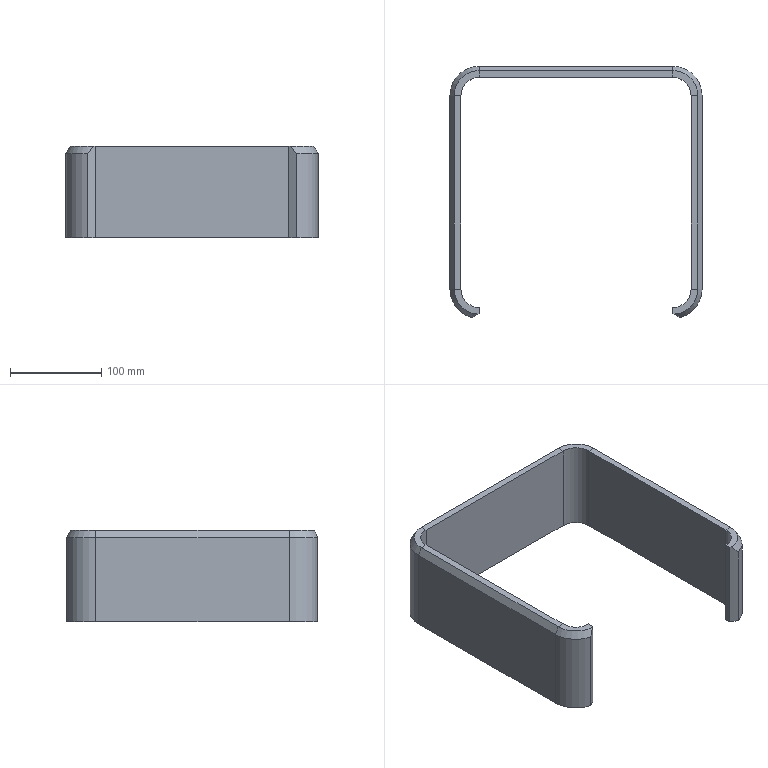Part | SolidWorks | features Chamfer 2, Extrusion 1, FlatPattern 1, RefAxis 1, SheetMetal 1, SolidToSheetMetal 1 | 1 solid | 39 faces | box 276 x 274.941 x 100 mm | volume 939173 mm3 | plane 27 | cylinder 8 | cone 4 | commonest cylinder face diameters 40 x4 64 x4
STEP:
#1=CARTESIAN_POINT('',(106.,-132.226,100.));
#2=VERTEX_POINT('',#1);
#3=CARTESIAN_POINT('',(106.,-126.,100.));
#4=VERTEX_POINT('',#3);
#5=CARTESIAN_POINT('',(106.,-126.,100.));
#6=DIRECTION('',(0.,1.,0.));
#7=VECTOR('',#6,1000.);
#8=LINE('',#5,#7);
#9=EDGE_CURVE('',#2,#4,#8,.T.);
#10=ORIENTED_EDGE('',*,*,#9,.F.);
#11=CARTESIAN_POINT('',(107.887,-133.316,100.));
#12=VERTEX_POINT('',#11);
#13=CARTESIAN_POINT('',(94.644,-125.67,100.));
#14=DIRECTION('',(0.866,-0.5,0.));
#15=VECTOR('',#14,1000.);
#16=LINE('',#13,#15);
#17=EDGE_CURVE('',#2,#12,#16,.T.);
#18=ORIENTED_EDGE('',*,*,#17,.T.);
#19=CARTESIAN_POINT('',(133.381,-106.,100.));
#20=VERTEX_POINT('',#19);
#21=CARTESIAN_POINT('',(106.,-106.,100.));
#22=DIRECTION('',(0.,0.,1.));
#23=DIRECTION('',(1.,0.,0.));
#24=AXIS2_PLACEMENT_3D('',#21,#22,#23);
#25=CIRCLE('',#24,27.381);
#26=EDGE_CURVE('',#12,#20,#25,.T.);
#27=ORIENTED_EDGE('',*,*,#26,.T.);
#28=CARTESIAN_POINT('',(126.,-106.,100.));
#29=VERTEX_POINT('',#28);
#30=CARTESIAN_POINT('',(126.,-106.,100.));
#31=DIRECTION('',(-1.,0.,0.));
#32=VECTOR('',#31,1000.);
#33=LINE('',#30,#32);
#34=EDGE_CURVE('',#20,#29,#33,.T.);
#35=ORIENTED_EDGE('',*,*,#34,.T.);
#36=CARTESIAN_POINT('',(106.,-106.,100.));
#37=DIRECTION('',(0.,0.,-1.));
#38=DIRECTION('',(1.,0.,0.));
#39=AXIS2_PLACEMENT_3D('',#36,#37,#38);
#40=CIRCLE('',#39,20.);
#41=EDGE_CURVE('',#29,#4,#40,.T.);
#42=ORIENTED_EDGE('',*,*,#41,.T.);
#43=EDGE_LOOP('',(#10,#18,#27,#35,#42));
#44=FACE_OUTER_BOUND('',#43,.T.);
#45=CARTESIAN_POINT('',(106.,-106.,100.));
#46=DIRECTION('',(0.,0.,1.));
#47=DIRECTION('',(1.,0.,0.));
#48=AXIS2_PLACEMENT_3D('',#45,#46,#47);
#49=PLANE('',#48);
#50=ADVANCED_FACE('',(#44),#49,.T.);
#51=ORIENTED_EDGE('',*,*,#34,.F.);
#52=CARTESIAN_POINT('',(133.381,106.,100.));
#53=VERTEX_POINT('',#52);
#54=CARTESIAN_POINT('',(133.381,106.,100.));
#55=DIRECTION('',(0.,1.,0.));
#56=VECTOR('',#55,1000.);
#57=LINE('',#54,#56);
#58=EDGE_CURVE('',#20,#53,#57,.T.);
#59=ORIENTED_EDGE('',*,*,#58,.T.);
#60=CARTESIAN_POINT('',(126.,106.,100.));
#61=VERTEX_POINT('',#60);
#62=CARTESIAN_POINT('',(126.,106.,100.));
#63=DIRECTION('',(-1.,0.,0.));
#64=VECTOR('',#63,1000.);
#65=LINE('',#62,#64);
#66=EDGE_CURVE('',#53,#61,#65,.T.);
#67=ORIENTED_EDGE('',*,*,#66,.T.);
#68=CARTESIAN_POINT('',(126.,106.,100.));
#69=DIRECTION('',(0.,-1.,0.));
#70=VECTOR('',#69,1000.);
#71=LINE('',#68,#70);
#72=EDGE_CURVE('',#61,#29,#71,.T.);
#73=ORIENTED_EDGE('',*,*,#72,.T.);
#74=EDGE_LOOP('',(#51,#59,#67,#73));
#75=FACE_OUTER_BOUND('',#74,.T.);
#76=CARTESIAN_POINT('',(126.,106.,100.));
#77=DIRECTION('',(0.,0.,1.));
#78=DIRECTION('',(0.,-1.,0.));
#79=AXIS2_PLACEMENT_3D('',#76,#77,#78);
#80=PLANE('',#79);
#81=ADVANCED_FACE('',(#75),#80,.T.);
#82=ORIENTED_EDGE('',*,*,#66,.F.);
#83=CARTESIAN_POINT('',(106.,133.381,100.));
#84=VERTEX_POINT('',#83);
#85=CARTESIAN_POINT('',(106.,106.,100.));
#86=DIRECTION('',(0.,0.,1.));
#87=DIRECTION('',(1.,0.,0.));
#88=AXIS2_PLACEMENT_3D('',#85,#86,#87);
#89=CIRCLE('',#88,27.381);
#90=EDGE_CURVE('',#53,#84,#89,.T.);
#91=ORIENTED_EDGE('',*,*,#90,.T.);
#92=CARTESIAN_POINT('',(106.,126.,100.));
#93=VERTEX_POINT('',#92);
#94=CARTESIAN_POINT('',(106.,126.,100.));
#95=DIRECTION('',(0.,-1.,0.));
#96=VECTOR('',#95,1000.);
#97=LINE('',#94,#96);
#98=EDGE_CURVE('',#84,#93,#97,.T.);
#99=ORIENTED_EDGE('',*,*,#98,.T.);
#100=CARTESIAN_POINT('',(106.,106.,100.));
#101=DIRECTION('',(0.,0.,-1.));
#102=DIRECTION('',(1.,0.,0.));
#103=AXIS2_PLACEMENT_3D('',#100,#101,#102);
#104=CIRCLE('',#103,20.);
#105=EDGE_CURVE('',#93,#61,#104,.T.);
#106=ORIENTED_EDGE('',*,*,#105,.T.);
#107=EDGE_LOOP('',(#82,#91,#99,#106));
#108=FACE_OUTER_BOUND('',#107,.T.);
#109=CARTESIAN_POINT('',(106.,106.,100.));
#110=DIRECTION('',(0.,0.,1.));
#111=DIRECTION('',(1.,0.,0.));
#112=AXIS2_PLACEMENT_3D('',#109,#110,#111);
#113=PLANE('',#112);
#114=ADVANCED_FACE('',(#108),#113,.T.);
#115=ORIENTED_EDGE('',*,*,#98,.F.);
#116=CARTESIAN_POINT('',(-106.,133.381,100.));
#117=VERTEX_POINT('',#116);
#118=CARTESIAN_POINT('',(-106.,133.381,100.));
#119=DIRECTION('',(-1.,0.,0.));
#120=VECTOR('',#119,1000.);
#121=LINE('',#118,#120);
#122=EDGE_CURVE('',#84,#117,#121,.T.);
#123=ORIENTED_EDGE('',*,*,#122,.T.);
#124=CARTESIAN_POINT('',(-106.,126.,100.));
#125=VERTEX_POINT('',#124);
#126=CARTESIAN_POINT('',(-106.,126.,100.));
#127=DIRECTION('',(0.,-1.,0.));
#128=VECTOR('',#127,1000.);
#129=LINE('',#126,#128);
#130=EDGE_CURVE('',#117,#125,#129,.T.);
#131=ORIENTED_EDGE('',*,*,#130,.T.);
#132=CARTESIAN_POINT('',(-106.,126.,100.));
#133=DIRECTION('',(1.,0.,0.));
#134=VECTOR('',#133,1000.);
#135=LINE('',#132,#134);
#136=EDGE_CURVE('',#125,#93,#135,.T.);
#137=ORIENTED_EDGE('',*,*,#136,.T.);
#138=EDGE_LOOP('',(#115,#123,#131,#137));
#139=FACE_OUTER_BOUND('',#138,.T.);
#140=CARTESIAN_POINT('',(-106.,126.,100.));
#141=DIRECTION('',(0.,0.,1.));
#142=DIRECTION('',(1.,0.,0.));
#143=AXIS2_PLACEMENT_3D('',#140,#141,#142);
#144=PLANE('',#143);
#145=ADVANCED_FACE('',(#139),#144,.T.);
#146=ORIENTED_EDGE('',*,*,#130,.F.);
#147=CARTESIAN_POINT('',(-133.381,106.,100.));
#148=VERTEX_POINT('',#147);
#149=CARTESIAN_POINT('',(-106.,106.,100.));
#150=DIRECTION('',(0.,0.,1.));
#151=DIRECTION('',(1.,0.,0.));
#152=AXIS2_PLACEMENT_3D('',#149,#150,#151);
#153=CIRCLE('',#152,27.381);
#154=EDGE_CURVE('',#117,#148,#153,.T.);
#155=ORIENTED_EDGE('',*,*,#154,.T.);
#156=CARTESIAN_POINT('',(-126.,106.,100.));
#157=VERTEX_POINT('',#156);
#158=CARTESIAN_POINT('',(-126.,106.,100.));
#159=DIRECTION('',(1.,0.,0.));
#160=VECTOR('',#159,1000.);
#161=LINE('',#158,#160);
#162=EDGE_CURVE('',#148,#157,#161,.T.);
#163=ORIENTED_EDGE('',*,*,#162,.T.);
#164=CARTESIAN_POINT('',(-106.,106.,100.));
#165=DIRECTION('',(0.,0.,-1.));
#166=DIRECTION('',(-1.,0.,0.));
#167=AXIS2_PLACEMENT_3D('',#164,#165,#166);
#168=CIRCLE('',#167,20.);
#169=EDGE_CURVE('',#157,#125,#168,.T.);
#170=ORIENTED_EDGE('',*,*,#169,.T.);
#171=EDGE_LOOP('',(#146,#155,#163,#170));
#172=FACE_OUTER_BOUND('',#171,.T.);
#173=CARTESIAN_POINT('',(-106.,106.,100.));
#174=DIRECTION('',(0.,0.,1.));
#175=DIRECTION('',(1.,0.,0.));
#176=AXIS2_PLACEMENT_3D('',#173,#174,#175);
#177=PLANE('',#176);
#178=ADVANCED_FACE('',(#172),#177,.T.);
#179=ORIENTED_EDGE('',*,*,#162,.F.);
#180=CARTESIAN_POINT('',(-133.381,-106.,100.));
#181=VERTEX_POINT('',#180);
#182=CARTESIAN_POINT('',(-133.381,-62.,100.));
#183=DIRECTION('',(0.,-1.,0.));
#184=VECTOR('',#183,1000.);
#185=LINE('',#182,#184);
#186=EDGE_CURVE('',#148,#181,#185,.T.);
#187=ORIENTED_EDGE('',*,*,#186,.T.);
#188=CARTESIAN_POINT('',(-126.,-106.,100.));
#189=VERTEX_POINT('',#188);
#190=CARTESIAN_POINT('',(-126.,-106.,100.));
#191=DIRECTION('',(1.,0.,0.));
#192=VECTOR('',#191,1000.);
#193=LINE('',#190,#192);
#194=EDGE_CURVE('',#181,#189,#193,.T.);
#195=ORIENTED_EDGE('',*,*,#194,.T.);
#196=CARTESIAN_POINT('',(-126.,-62.,100.));
#197=DIRECTION('',(0.,1.,0.));
#198=VECTOR('',#197,1000.);
#199=LINE('',#196,#198);
#200=EDGE_CURVE('',#189,#157,#199,.T.);
#201=ORIENTED_EDGE('',*,*,#200,.T.);
#202=EDGE_LOOP('',(#179,#187,#195,#201));
#203=FACE_OUTER_BOUND('',#202,.T.);
#204=CARTESIAN_POINT('',(-126.,-62.,100.));
#205=DIRECTION('',(0.,0.,1.));
#206=DIRECTION('',(0.,1.,0.));
#207=AXIS2_PLACEMENT_3D('',#204,#205,#206);
#208=PLANE('',#207);
#209=ADVANCED_FACE('',(#203),#208,.T.);
#210=CARTESIAN_POINT('',(-107.887,-133.316,100.));
#211=VERTEX_POINT('',#210);
#212=CARTESIAN_POINT('',(-106.,-106.,100.));
#213=DIRECTION('',(0.,0.,1.));
#214=DIRECTION('',(1.,0.,0.));
#215=AXIS2_PLACEMENT_3D('',#212,#213,#214);
#216=CIRCLE('',#215,27.381);
#217=EDGE_CURVE('',#181,#211,#216,.T.);
#218=ORIENTED_EDGE('',*,*,#217,.T.);
#219=CARTESIAN_POINT('',(-106.,-132.226,100.));
#220=VERTEX_POINT('',#219);
#221=CARTESIAN_POINT('',(-94.644,-125.67,100.));
#222=DIRECTION('',(0.866,0.5,0.));
#223=VECTOR('',#222,1000.);
#224=LINE('',#221,#223);
#225=EDGE_CURVE('',#211,#220,#224,.T.);
#226=ORIENTED_EDGE('',*,*,#225,.T.);
#227=CARTESIAN_POINT('',(-106.,-126.,100.));
#228=VERTEX_POINT('',#227);
#229=CARTESIAN_POINT('',(-106.,-126.,100.));
#230=DIRECTION('',(0.,1.,0.));
#231=VECTOR('',#230,1000.);
#232=LINE('',#229,#231);
#233=EDGE_CURVE('',#220,#228,#232,.T.);
#234=ORIENTED_EDGE('',*,*,#233,.T.);
#235=CARTESIAN_POINT('',(-106.,-106.,100.));
#236=DIRECTION('',(0.,0.,-1.));
#237=DIRECTION('',(-1.,0.,0.));
#238=AXIS2_PLACEMENT_3D('',#235,#236,#237);
#239=CIRCLE('',#238,20.);
#240=EDGE_CURVE('',#228,#189,#239,.T.);
#241=ORIENTED_EDGE('',*,*,#240,.T.);
#242=ORIENTED_EDGE('',*,*,#194,.F.);
#243=EDGE_LOOP('',(#218,#226,#234,#241,#242));
#244=FACE_OUTER_BOUND('',#243,.T.);
#245=CARTESIAN_POINT('',(-106.,-106.,100.));
#246=DIRECTION('',(0.,0.,1.));
#247=DIRECTION('',(1.,0.,0.));
#248=AXIS2_PLACEMENT_3D('',#245,#246,#247);
#249=PLANE('',#248);
#250=ADVANCED_FACE('',(#244),#249,.T.);
#251=ORIENTED_EDGE('',*,*,#233,.F.);
#252=CARTESIAN_POINT('',(-106.,-132.226,0.));
#253=VERTEX_POINT('',#252);
#254=CARTESIAN_POINT('',(-106.,-132.226,50.));
#255=DIRECTION('',(0.,0.,-1.));
#256=VECTOR('',#255,1000.);
#257=LINE('',#254,#256);
#258=EDGE_CURVE('',#220,#253,#257,.T.);
#259=ORIENTED_EDGE('',*,*,#258,.T.);
#260=CARTESIAN_POINT('',(-106.,-126.,0.));
#261=VERTEX_POINT('',#260);
#262=CARTESIAN_POINT('',(-106.,-126.,0.));
#263=DIRECTION('',(0.,1.,0.));
#264=VECTOR('',#263,1000.);
#265=LINE('',#262,#264);
#266=EDGE_CURVE('',#253,#261,#265,.T.);
#267=ORIENTED_EDGE('',*,*,#266,.T.);
#268=CARTESIAN_POINT('',(-106.,-126.,100.));
#269=DIRECTION('',(0.,0.,-1.));
#270=VECTOR('',#269,1000.);
#271=LINE('',#268,#270);
#272=EDGE_CURVE('',#228,#261,#271,.T.);
#273=ORIENTED_EDGE('',*,*,#272,.F.);
#274=EDGE_LOOP('',(#251,#259,#267,#273));
#275=FACE_OUTER_BOUND('',#274,.T.);
#276=CARTESIAN_POINT('',(-106.,-126.,50.));
#277=DIRECTION('',(-1.,0.,0.));
#278=DIRECTION('',(0.,0.,-1.));
#279=AXIS2_PLACEMENT_3D('',#276,#277,#278);
#280=PLANE('',#279);
#281=ADVANCED_FACE('',(#275),#280,.F.);
#282=ORIENTED_EDGE('',*,*,#266,.F.);
#283=CARTESIAN_POINT('',(-114.165,-136.941,0.));
#284=VERTEX_POINT('',#283);
#285=CARTESIAN_POINT('',(-94.644,-125.67,0.));
#286=DIRECTION('',(-0.866,-0.5,0.));
#287=VECTOR('',#286,1000.);
#288=LINE('',#285,#287);
#289=EDGE_CURVE('',#253,#284,#288,.T.);
#290=ORIENTED_EDGE('',*,*,#289,.T.);
#291=CARTESIAN_POINT('',(-138.,-106.,0.));
#292=VERTEX_POINT('',#291);
#293=CARTESIAN_POINT('',(-106.,-106.,0.));
#294=DIRECTION('',(0.,0.,-1.));
#295=DIRECTION('',(-1.,0.,0.));
#296=AXIS2_PLACEMENT_3D('',#293,#294,#295);
#297=CIRCLE('',#296,32.);
#298=EDGE_CURVE('',#284,#292,#297,.T.);
#299=ORIENTED_EDGE('',*,*,#298,.T.);
#300=CARTESIAN_POINT('',(-126.,-106.,0.));
#301=VERTEX_POINT('',#300);
#302=CARTESIAN_POINT('',(-126.,-106.,0.));
#303=DIRECTION('',(1.,0.,0.));
#304=VECTOR('',#303,1000.);
#305=LINE('',#302,#304);
#306=EDGE_CURVE('',#292,#301,#305,.T.);
#307=ORIENTED_EDGE('',*,*,#306,.T.);
#308=CARTESIAN_POINT('',(-106.,-106.,0.));
#309=DIRECTION('',(0.,0.,-1.));
#310=DIRECTION('',(-1.,0.,0.));
#311=AXIS2_PLACEMENT_3D('',#308,#309,#310);
#312=CIRCLE('',#311,20.);
#313=EDGE_CURVE('',#261,#301,#312,.T.);
#314=ORIENTED_EDGE('',*,*,#313,.F.);
#315=EDGE_LOOP('',(#282,#290,#299,#307,#314));
#316=FACE_OUTER_BOUND('',#315,.T.);
#317=CARTESIAN_POINT('',(-106.,-106.,0.));
#318=DIRECTION('',(0.,0.,1.));
#319=DIRECTION('',(1.,0.,0.));
#320=AXIS2_PLACEMENT_3D('',#317,#318,#319);
#321=PLANE('',#320);
#322=ADVANCED_FACE('',(#316),#321,.F.);
#323=ORIENTED_EDGE('',*,*,#306,.F.);
#324=CARTESIAN_POINT('',(-138.,106.,0.));
#325=VERTEX_POINT('',#324);
#326=CARTESIAN_POINT('',(-138.,106.,0.));
#327=DIRECTION('',(0.,1.,0.));
#328=VECTOR('',#327,1000.);
#329=LINE('',#326,#328);
#330=EDGE_CURVE('',#292,#325,#329,.T.);
#331=ORIENTED_EDGE('',*,*,#330,.T.);
#332=CARTESIAN_POINT('',(-126.,106.,0.));
#333=VERTEX_POINT('',#332);
#334=CARTESIAN_POINT('',(-126.,106.,0.));
#335=DIRECTION('',(1.,0.,0.));
#336=VECTOR('',#335,1000.);
#337=LINE('',#334,#336);
#338=EDGE_CURVE('',#325,#333,#337,.T.);
#339=ORIENTED_EDGE('',*,*,#338,.T.);
#340=CARTESIAN_POINT('',(-126.,106.,0.));
#341=DIRECTION('',(0.,1.,0.));
#342=VECTOR('',#341,1000.);
#343=LINE('',#340,#342);
#344=EDGE_CURVE('',#301,#333,#343,.T.);
#345=ORIENTED_EDGE('',*,*,#344,.F.);
#346=EDGE_LOOP('',(#323,#331,#339,#345));
#347=FACE_OUTER_BOUND('',#346,.T.);
#348=CARTESIAN_POINT('',(-126.,106.,0.));
#349=DIRECTION('',(0.,0.,1.));
#350=DIRECTION('',(0.,1.,0.));
#351=AXIS2_PLACEMENT_3D('',#348,#349,#350);
#352=PLANE('',#351);
#353=ADVANCED_FACE('',(#347),#352,.F.);
#354=ORIENTED_EDGE('',*,*,#338,.F.);
#355=CARTESIAN_POINT('',(-106.,138.,0.));
#356=VERTEX_POINT('',#355);
#357=CARTESIAN_POINT('',(-106.,106.,0.));
#358=DIRECTION('',(0.,0.,-1.));
#359=DIRECTION('',(-1.,0.,0.));
#360=AXIS2_PLACEMENT_3D('',#357,#358,#359);
#361=CIRCLE('',#360,32.);
#362=EDGE_CURVE('',#325,#356,#361,.T.);
#363=ORIENTED_EDGE('',*,*,#362,.T.);
#364=CARTESIAN_POINT('',(-106.,126.,0.));
#365=VERTEX_POINT('',#364);
#366=CARTESIAN_POINT('',(-106.,126.,0.));
#367=DIRECTION('',(0.,-1.,0.));
#368=VECTOR('',#367,1000.);
#369=LINE('',#366,#368);
#370=EDGE_CURVE('',#356,#365,#369,.T.);
#371=ORIENTED_EDGE('',*,*,#370,.T.);
#372=CARTESIAN_POINT('',(-106.,106.,0.));
#373=DIRECTION('',(0.,0.,-1.));
#374=DIRECTION('',(-1.,0.,0.));
#375=AXIS2_PLACEMENT_3D('',#372,#373,#374);
#376=CIRCLE('',#375,20.);
#377=EDGE_CURVE('',#333,#365,#376,.T.);
#378=ORIENTED_EDGE('',*,*,#377,.F.);
#379=EDGE_LOOP('',(#354,#363,#371,#378));
#380=FACE_OUTER_BOUND('',#379,.T.);
#381=CARTESIAN_POINT('',(-106.,106.,0.));
#382=DIRECTION('',(0.,0.,1.));
#383=DIRECTION('',(1.,0.,0.));
#384=AXIS2_PLACEMENT_3D('',#381,#382,#383);
#385=PLANE('',#384);
#386=ADVANCED_FACE('',(#380),#385,.F.);
#387=ORIENTED_EDGE('',*,*,#370,.F.);
#388=CARTESIAN_POINT('',(106.,138.,0.));
#389=VERTEX_POINT('',#388);
#390=CARTESIAN_POINT('',(-106.,138.,0.));
#391=DIRECTION('',(1.,0.,0.));
#392=VECTOR('',#391,1000.);
#393=LINE('',#390,#392);
#394=EDGE_CURVE('',#356,#389,#393,.T.);
#395=ORIENTED_EDGE('',*,*,#394,.T.);
#396=CARTESIAN_POINT('',(106.,126.,0.));
#397=VERTEX_POINT('',#396);
#398=CARTESIAN_POINT('',(106.,126.,0.));
#399=DIRECTION('',(0.,-1.,0.));
#400=VECTOR('',#399,1000.);
#401=LINE('',#398,#400);
#402=EDGE_CURVE('',#389,#397,#401,.T.);
#403=ORIENTED_EDGE('',*,*,#402,.T.);
#404=CARTESIAN_POINT('',(-106.,126.,0.));
#405=DIRECTION('',(1.,0.,0.));
#406=VECTOR('',#405,1000.);
#407=LINE('',#404,#406);
#408=EDGE_CURVE('',#365,#397,#407,.T.);
#409=ORIENTED_EDGE('',*,*,#408,.F.);
#410=EDGE_LOOP('',(#387,#395,#403,#409));
#411=FACE_OUTER_BOUND('',#410,.T.);
#412=CARTESIAN_POINT('',(-106.,126.,0.));
#413=DIRECTION('',(0.,0.,1.));
#414=DIRECTION('',(1.,0.,0.));
#415=AXIS2_PLACEMENT_3D('',#412,#413,#414);
#416=PLANE('',#415);
#417=ADVANCED_FACE('',(#411),#416,.F.);
#418=ORIENTED_EDGE('',*,*,#402,.F.);
#419=CARTESIAN_POINT('',(138.,106.,0.));
#420=VERTEX_POINT('',#419);
#421=CARTESIAN_POINT('',(106.,106.,0.));
#422=DIRECTION('',(0.,0.,-1.));
#423=DIRECTION('',(-1.,0.,0.));
#424=AXIS2_PLACEMENT_3D('',#421,#422,#423);
#425=CIRCLE('',#424,32.);
#426=EDGE_CURVE('',#389,#420,#425,.T.);
#427=ORIENTED_EDGE('',*,*,#426,.T.);
#428=CARTESIAN_POINT('',(126.,106.,0.));
#429=VERTEX_POINT('',#428);
#430=CARTESIAN_POINT('',(126.,106.,0.));
#431=DIRECTION('',(-1.,0.,0.));
#432=VECTOR('',#431,1000.);
#433=LINE('',#430,#432);
#434=EDGE_CURVE('',#420,#429,#433,.T.);
#435=ORIENTED_EDGE('',*,*,#434,.T.);
#436=CARTESIAN_POINT('',(106.,106.,0.));
#437=DIRECTION('',(0.,0.,-1.));
#438=DIRECTION('',(1.,0.,0.));
#439=AXIS2_PLACEMENT_3D('',#436,#437,#438);
#440=CIRCLE('',#439,20.);
#441=EDGE_CURVE('',#397,#429,#440,.T.);
#442=ORIENTED_EDGE('',*,*,#441,.F.);
#443=EDGE_LOOP('',(#418,#427,#435,#442));
#444=FACE_OUTER_BOUND('',#443,.T.);
#445=CARTESIAN_POINT('',(106.,106.,0.));
#446=DIRECTION('',(0.,0.,1.));
#447=DIRECTION('',(1.,0.,0.));
#448=AXIS2_PLACEMENT_3D('',#445,#446,#447);
#449=PLANE('',#448);
#450=ADVANCED_FACE('',(#444),#449,.F.);
#451=ORIENTED_EDGE('',*,*,#434,.F.);
#452=CARTESIAN_POINT('',(138.,-106.,0.));
#453=VERTEX_POINT('',#452);
#454=CARTESIAN_POINT('',(138.,-106.,0.));
#455=DIRECTION('',(0.,-1.,0.));
#456=VECTOR('',#455,1000.);
#457=LINE('',#454,#456);
#458=EDGE_CURVE('',#420,#453,#457,.T.);
#459=ORIENTED_EDGE('',*,*,#458,.T.);
#460=CARTESIAN_POINT('',(126.,-106.,0.));
#461=VERTEX_POINT('',#460);
#462=CARTESIAN_POINT('',(126.,-106.,0.));
#463=DIRECTION('',(-1.,0.,0.));
#464=VECTOR('',#463,1000.);
#465=LINE('',#462,#464);
#466=EDGE_CURVE('',#453,#461,#465,.T.);
#467=ORIENTED_EDGE('',*,*,#466,.T.);
#468=CARTESIAN_POINT('',(126.,-106.,0.));
#469=DIRECTION('',(0.,-1.,0.));
#470=VECTOR('',#469,1000.);
#471=LINE('',#468,#470);
#472=EDGE_CURVE('',#429,#461,#471,.T.);
#473=ORIENTED_EDGE('',*,*,#472,.F.);
#474=EDGE_LOOP('',(#451,#459,#467,#473));
#475=FACE_OUTER_BOUND('',#474,.T.);
#476=CARTESIAN_POINT('',(126.,-106.,0.));
#477=DIRECTION('',(0.,0.,1.));
#478=DIRECTION('',(0.,-1.,0.));
#479=AXIS2_PLACEMENT_3D('',#476,#477,#478);
#480=PLANE('',#479);
#481=ADVANCED_FACE('',(#475),#480,.F.);
#482=CARTESIAN_POINT('',(114.165,-136.941,0.));
#483=VERTEX_POINT('',#482);
#484=CARTESIAN_POINT('',(106.,-106.,0.));
#485=DIRECTION('',(0.,0.,-1.));
#486=DIRECTION('',(-1.,0.,0.));
#487=AXIS2_PLACEMENT_3D('',#484,#485,#486);
#488=CIRCLE('',#487,32.);
#489=EDGE_CURVE('',#453,#483,#488,.T.);
#490=ORIENTED_EDGE('',*,*,#489,.T.);
#491=CARTESIAN_POINT('',(106.,-132.226,0.));
#492=VERTEX_POINT('',#491);
#493=CARTESIAN_POINT('',(94.644,-125.67,0.));
#494=DIRECTION('',(-0.866,0.5,0.));
#495=VECTOR('',#494,1000.);
#496=LINE('',#493,#495);
#497=EDGE_CURVE('',#483,#492,#496,.T.);
#498=ORIENTED_EDGE('',*,*,#497,.T.);
#499=CARTESIAN_POINT('',(106.,-126.,0.));
#500=VERTEX_POINT('',#499);
#501=CARTESIAN_POINT('',(106.,-126.,0.));
#502=DIRECTION('',(0.,1.,0.));
#503=VECTOR('',#502,1000.);
#504=LINE('',#501,#503);
#505=EDGE_CURVE('',#492,#500,#504,.T.);
#506=ORIENTED_EDGE('',*,*,#505,.T.);
#507=CARTESIAN_POINT('',(106.,-106.,0.));
#508=DIRECTION('',(0.,0.,-1.));
#509=DIRECTION('',(1.,0.,0.));
#510=AXIS2_PLACEMENT_3D('',#507,#508,#509);
#511=CIRCLE('',#510,20.);
#512=EDGE_CURVE('',#461,#500,#511,.T.);
#513=ORIENTED_EDGE('',*,*,#512,.F.);
#514=ORIENTED_EDGE('',*,*,#466,.F.);
#515=EDGE_LOOP('',(#490,#498,#506,#513,#514));
#516=FACE_OUTER_BOUND('',#515,.T.);
#517=CARTESIAN_POINT('',(106.,-106.,0.));
#518=DIRECTION('',(0.,0.,1.));
#519=DIRECTION('',(1.,0.,0.));
#520=AXIS2_PLACEMENT_3D('',#517,#518,#519);
#521=PLANE('',#520);
#522=ADVANCED_FACE('',(#516),#521,.F.);
#523=ORIENTED_EDGE('',*,*,#505,.F.);
#524=CARTESIAN_POINT('',(106.,-132.226,50.));
#525=DIRECTION('',(0.,0.,1.));
#526=VECTOR('',#525,1000.);
#527=LINE('',#524,#526);
#528=EDGE_CURVE('',#492,#2,#527,.T.);
#529=ORIENTED_EDGE('',*,*,#528,.T.);
#530=ORIENTED_EDGE('',*,*,#9,.T.);
#531=CARTESIAN_POINT('',(106.,-126.,100.));
#532=DIRECTION('',(0.,0.,-1.));
#533=VECTOR('',#532,1000.);
#534=LINE('',#531,#533);
#535=EDGE_CURVE('',#4,#500,#534,.T.);
#536=ORIENTED_EDGE('',*,*,#535,.T.);
#537=EDGE_LOOP('',(#523,#529,#530,#536));
#538=FACE_OUTER_BOUND('',#537,.T.);
#539=CARTESIAN_POINT('',(106.,-126.,50.));
#540=DIRECTION('',(-1.,0.,0.));
#541=DIRECTION('',(0.,0.,-1.));
#542=AXIS2_PLACEMENT_3D('',#539,#540,#541);
#543=PLANE('',#542);
#544=ADVANCED_FACE('',(#538),#543,.T.);
#545=ORIENTED_EDGE('',*,*,#512,.T.);
#546=ORIENTED_EDGE('',*,*,#535,.F.);
#547=ORIENTED_EDGE('',*,*,#41,.F.);
#548=CARTESIAN_POINT('',(126.,-106.,100.));
#549=DIRECTION('',(0.,0.,-1.));
#550=VECTOR('',#549,1000.);
#551=LINE('',#548,#550);
#552=EDGE_CURVE('',#29,#461,#551,.T.);
#553=ORIENTED_EDGE('',*,*,#552,.T.);
#554=EDGE_LOOP('',(#545,#546,#547,#553));
#555=FACE_OUTER_BOUND('',#554,.T.);
#556=CARTESIAN_POINT('',(106.,-106.,100.));
#557=DIRECTION('',(0.,0.,-1.));
#558=DIRECTION('',(-1.,0.,0.));
#559=AXIS2_PLACEMENT_3D('',#556,#557,#558);
#560=CYLINDRICAL_SURFACE('',#559,20.);
#561=ADVANCED_FACE('',(#555),#560,.F.);
#562=ORIENTED_EDGE('',*,*,#313,.T.);
#563=CARTESIAN_POINT('',(-126.,-106.,100.));
#564=DIRECTION('',(0.,0.,-1.));
#565=VECTOR('',#564,1000.);
#566=LINE('',#563,#565);
#567=EDGE_CURVE('',#189,#301,#566,.T.);
#568=ORIENTED_EDGE('',*,*,#567,.F.);
#569=ORIENTED_EDGE('',*,*,#240,.F.);
#570=ORIENTED_EDGE('',*,*,#272,.T.);
#571=EDGE_LOOP('',(#562,#568,#569,#570));
#572=FACE_OUTER_BOUND('',#571,.T.);
#573=CARTESIAN_POINT('',(-106.,-106.,100.));
#574=DIRECTION('',(0.,0.,-1.));
#575=DIRECTION('',(-1.,0.,0.));
#576=AXIS2_PLACEMENT_3D('',#573,#574,#575);
#577=CYLINDRICAL_SURFACE('',#576,20.);
#578=ADVANCED_FACE('',(#572),#577,.F.);
#579=ORIENTED_EDGE('',*,*,#377,.T.);
#580=CARTESIAN_POINT('',(-106.,126.,100.));
#581=DIRECTION('',(0.,0.,-1.));
#582=VECTOR('',#581,1000.);
#583=LINE('',#580,#582);
#584=EDGE_CURVE('',#125,#365,#583,.T.);
#585=ORIENTED_EDGE('',*,*,#584,.F.);
#586=ORIENTED_EDGE('',*,*,#169,.F.);
#587=CARTESIAN_POINT('',(-126.,106.,100.));
#588=DIRECTION('',(0.,0.,-1.));
#589=VECTOR('',#588,1000.);
#590=LINE('',#587,#589);
#591=EDGE_CURVE('',#157,#333,#590,.T.);
#592=ORIENTED_EDGE('',*,*,#591,.T.);
#593=EDGE_LOOP('',(#579,#585,#586,#592));
#594=FACE_OUTER_BOUND('',#593,.T.);
#595=CARTESIAN_POINT('',(-106.,106.,100.));
#596=DIRECTION('',(0.,0.,-1.));
#597=DIRECTION('',(-1.,0.,0.));
#598=AXIS2_PLACEMENT_3D('',#595,#596,#597);
#599=CYLINDRICAL_SURFACE('',#598,20.);
#600=ADVANCED_FACE('',(#594),#599,.F.);
#601=ORIENTED_EDGE('',*,*,#344,.T.);
#602=ORIENTED_EDGE('',*,*,#591,.F.);
#603=ORIENTED_EDGE('',*,*,#200,.F.);
#604=ORIENTED_EDGE('',*,*,#567,.T.);
#605=EDGE_LOOP('',(#601,#602,#603,#604));
#606=FACE_OUTER_BOUND('',#605,.T.);
#607=CARTESIAN_POINT('',(-126.,106.,100.));
#608=DIRECTION('',(-1.,0.,0.));
#609=DIRECTION('',(0.,-1.,0.));
#610=AXIS2_PLACEMENT_3D('',#607,#608,#609);
#611=PLANE('',#610);
#612=ADVANCED_FACE('',(#606),#611,.F.);
#613=ORIENTED_EDGE('',*,*,#441,.T.);
#614=CARTESIAN_POINT('',(126.,106.,100.));
#615=DIRECTION('',(0.,0.,-1.));
#616=VECTOR('',#615,1000.);
#617=LINE('',#614,#616);
#618=EDGE_CURVE('',#61,#429,#617,.T.);
#619=ORIENTED_EDGE('',*,*,#618,.F.);
#620=ORIENTED_EDGE('',*,*,#105,.F.);
#621=CARTESIAN_POINT('',(106.,126.,100.));
#622=DIRECTION('',(0.,0.,-1.));
#623=VECTOR('',#622,1000.);
#624=LINE('',#621,#623);
#625=EDGE_CURVE('',#93,#397,#624,.T.);
#626=ORIENTED_EDGE('',*,*,#625,.T.);
#627=EDGE_LOOP('',(#613,#619,#620,#626));
#628=FACE_OUTER_BOUND('',#627,.T.);
#629=CARTESIAN_POINT('',(106.,106.,100.));
#630=DIRECTION('',(0.,0.,-1.));
#631=DIRECTION('',(-1.,0.,0.));
#632=AXIS2_PLACEMENT_3D('',#629,#630,#631);
#633=CYLINDRICAL_SURFACE('',#632,20.);
#634=ADVANCED_FACE('',(#628),#633,.F.);
#635=ORIENTED_EDGE('',*,*,#408,.T.);
#636=ORIENTED_EDGE('',*,*,#625,.F.);
#637=ORIENTED_EDGE('',*,*,#136,.F.);
#638=ORIENTED_EDGE('',*,*,#584,.T.);
#639=EDGE_LOOP('',(#635,#636,#637,#638));
#640=FACE_OUTER_BOUND('',#639,.T.);
#641=CARTESIAN_POINT('',(-106.,126.,100.));
#642=DIRECTION('',(0.,1.,0.));
#643=DIRECTION('',(0.,0.,1.));
#644=AXIS2_PLACEMENT_3D('',#641,#642,#643);
#645=PLANE('',#644);
#646=ADVANCED_FACE('',(#640),#645,.F.);
#647=ORIENTED_EDGE('',*,*,#472,.T.);
#648=ORIENTED_EDGE('',*,*,#552,.F.);
#649=ORIENTED_EDGE('',*,*,#72,.F.);
#650=ORIENTED_EDGE('',*,*,#618,.T.);
#651=EDGE_LOOP('',(#647,#648,#649,#650));
#652=FACE_OUTER_BOUND('',#651,.T.);
#653=CARTESIAN_POINT('',(126.,-106.,100.));
#654=DIRECTION('',(1.,0.,0.));
#655=DIRECTION('',(0.,1.,0.));
#656=AXIS2_PLACEMENT_3D('',#653,#654,#655);
#657=PLANE('',#656);
#658=ADVANCED_FACE('',(#652),#657,.F.);
#659=CARTESIAN_POINT('',(138.,-106.,92.));
#660=VERTEX_POINT('',#659);
#661=CARTESIAN_POINT('',(114.165,-136.941,92.));
#662=VERTEX_POINT('',#661);
#663=CARTESIAN_POINT('',(106.,-106.,92.));
#664=DIRECTION('',(0.,0.,-1.));
#665=DIRECTION('',(1.,0.,0.));
#666=AXIS2_PLACEMENT_3D('',#663,#664,#665);
#667=CIRCLE('',#666,32.);
#668=EDGE_CURVE('',#660,#662,#667,.T.);
#669=ORIENTED_EDGE('',*,*,#668,.T.);
#670=CARTESIAN_POINT('',(114.165,-136.941,100.));
#671=DIRECTION('',(0.,0.,-1.));
#672=VECTOR('',#671,1000.);
#673=LINE('',#670,#672);
#674=EDGE_CURVE('',#662,#483,#673,.T.);
#675=ORIENTED_EDGE('',*,*,#674,.T.);
#676=ORIENTED_EDGE('',*,*,#489,.F.);
#677=CARTESIAN_POINT('',(138.,-106.,100.));
#678=DIRECTION('',(0.,0.,-1.));
#679=VECTOR('',#678,1000.);
#680=LINE('',#677,#679);
#681=EDGE_CURVE('',#660,#453,#680,.T.);
#682=ORIENTED_EDGE('',*,*,#681,.F.);
#683=EDGE_LOOP('',(#669,#675,#676,#682));
#684=FACE_OUTER_BOUND('',#683,.T.);
#685=CARTESIAN_POINT('',(106.,-106.,100.));
#686=DIRECTION('',(0.,0.,-1.));
#687=DIRECTION('',(-1.,0.,0.));
#688=AXIS2_PLACEMENT_3D('',#685,#686,#687);
#689=CYLINDRICAL_SURFACE('',#688,32.);
#690=ADVANCED_FACE('',(#684),#689,.T.);
#691=ORIENTED_EDGE('',*,*,#298,.F.);
#692=CARTESIAN_POINT('',(-114.165,-136.941,92.));
#693=VERTEX_POINT('',#692);
#694=CARTESIAN_POINT('',(-114.165,-136.941,100.));
#695=DIRECTION('',(0.,0.,1.));
#696=VECTOR('',#695,1000.);
#697=LINE('',#694,#696);
#698=EDGE_CURVE('',#284,#693,#697,.T.);
#699=ORIENTED_EDGE('',*,*,#698,.T.);
#700=CARTESIAN_POINT('',(-138.,-106.,92.));
#701=VERTEX_POINT('',#700);
#702=CARTESIAN_POINT('',(-106.,-106.,92.));
#703=DIRECTION('',(0.,0.,-1.));
#704=DIRECTION('',(1.,0.,0.));
#705=AXIS2_PLACEMENT_3D('',#702,#703,#704);
#706=CIRCLE('',#705,32.);
#707=EDGE_CURVE('',#693,#701,#706,.T.);
#708=ORIENTED_EDGE('',*,*,#707,.T.);
#709=CARTESIAN_POINT('',(-138.,-106.,100.));
#710=DIRECTION('',(0.,0.,-1.));
#711=VECTOR('',#710,1000.);
#712=LINE('',#709,#711);
#713=EDGE_CURVE('',#701,#292,#712,.T.);
#714=ORIENTED_EDGE('',*,*,#713,.T.);
#715=EDGE_LOOP('',(#691,#699,#708,#714));
#716=FACE_OUTER_BOUND('',#715,.T.);
#717=CARTESIAN_POINT('',(-106.,-106.,100.));
#718=DIRECTION('',(0.,0.,-1.));
#719=DIRECTION('',(-1.,0.,0.));
#720=AXIS2_PLACEMENT_3D('',#717,#718,#719);
#721=CYLINDRICAL_SURFACE('',#720,32.);
#722=ADVANCED_FACE('',(#716),#721,.T.);
#723=CARTESIAN_POINT('',(-138.,106.,92.));
#724=VERTEX_POINT('',#723);
#725=CARTESIAN_POINT('',(-138.,106.,100.));
#726=DIRECTION('',(0.,0.,-1.));
#727=VECTOR('',#726,1000.);
#728=LINE('',#725,#727);
#729=EDGE_CURVE('',#724,#325,#728,.T.);
#730=ORIENTED_EDGE('',*,*,#729,.F.);
#731=CARTESIAN_POINT('',(-106.,138.,92.));
#732=VERTEX_POINT('',#731);
#733=CARTESIAN_POINT('',(-106.,106.,92.));
#734=DIRECTION('',(0.,0.,-1.));
#735=DIRECTION('',(1.,0.,0.));
#736=AXIS2_PLACEMENT_3D('',#733,#734,#735);
#737=CIRCLE('',#736,32.);
#738=EDGE_CURVE('',#724,#732,#737,.T.);
#739=ORIENTED_EDGE('',*,*,#738,.T.);
#740=CARTESIAN_POINT('',(-106.,138.,100.));
#741=DIRECTION('',(0.,0.,-1.));
#742=VECTOR('',#741,1000.);
#743=LINE('',#740,#742);
#744=EDGE_CURVE('',#732,#356,#743,.T.);
#745=ORIENTED_EDGE('',*,*,#744,.T.);
#746=ORIENTED_EDGE('',*,*,#362,.F.);
#747=EDGE_LOOP('',(#730,#739,#745,#746));
#748=FACE_OUTER_BOUND('',#747,.T.);
#749=CARTESIAN_POINT('',(-106.,106.,100.));
#750=DIRECTION('',(0.,0.,-1.));
#751=DIRECTION('',(-1.,0.,0.));
#752=AXIS2_PLACEMENT_3D('',#749,#750,#751);
#753=CYLINDRICAL_SURFACE('',#752,32.);
#754=ADVANCED_FACE('',(#748),#753,.T.);
#755=ORIENTED_EDGE('',*,*,#713,.F.);
#756=CARTESIAN_POINT('',(-138.,106.,92.));
#757=DIRECTION('',(0.,1.,0.));
#758=VECTOR('',#757,1000.);
#759=LINE('',#756,#758);
#760=EDGE_CURVE('',#701,#724,#759,.T.);
#761=ORIENTED_EDGE('',*,*,#760,.T.);
#762=ORIENTED_EDGE('',*,*,#729,.T.);
#763=ORIENTED_EDGE('',*,*,#330,.F.);
#764=EDGE_LOOP('',(#755,#761,#762,#763));
#765=FACE_OUTER_BOUND('',#764,.T.);
#766=CARTESIAN_POINT('',(-138.,106.,100.));
#767=DIRECTION('',(-1.,0.,0.));
#768=DIRECTION('',(0.,-1.,0.));
#769=AXIS2_PLACEMENT_3D('',#766,#767,#768);
#770=PLANE('',#769);
#771=ADVANCED_FACE('',(#765),#770,.T.);
#772=CARTESIAN_POINT('',(106.,138.,92.));
#773=VERTEX_POINT('',#772);
#774=CARTESIAN_POINT('',(106.,138.,100.));
#775=DIRECTION('',(0.,0.,-1.));
#776=VECTOR('',#775,1000.);
#777=LINE('',#774,#776);
#778=EDGE_CURVE('',#773,#389,#777,.T.);
#779=ORIENTED_EDGE('',*,*,#778,.F.);
#780=CARTESIAN_POINT('',(138.,106.,92.));
#781=VERTEX_POINT('',#780);
#782=CARTESIAN_POINT('',(106.,106.,92.));
#783=DIRECTION('',(0.,0.,-1.));
#784=DIRECTION('',(1.,0.,0.));
#785=AXIS2_PLACEMENT_3D('',#782,#783,#784);
#786=CIRCLE('',#785,32.);
#787=EDGE_CURVE('',#773,#781,#786,.T.);
#788=ORIENTED_EDGE('',*,*,#787,.T.);
#789=CARTESIAN_POINT('',(138.,106.,100.));
#790=DIRECTION('',(0.,0.,-1.));
#791=VECTOR('',#790,1000.);
#792=LINE('',#789,#791);
#793=EDGE_CURVE('',#781,#420,#792,.T.);
#794=ORIENTED_EDGE('',*,*,#793,.T.);
#795=ORIENTED_EDGE('',*,*,#426,.F.);
#796=EDGE_LOOP('',(#779,#788,#794,#795));
#797=FACE_OUTER_BOUND('',#796,.T.);
#798=CARTESIAN_POINT('',(106.,106.,100.));
#799=DIRECTION('',(0.,0.,-1.));
#800=DIRECTION('',(-1.,0.,0.));
#801=AXIS2_PLACEMENT_3D('',#798,#799,#800);
#802=CYLINDRICAL_SURFACE('',#801,32.);
#803=ADVANCED_FACE('',(#797),#802,.T.);
#804=ORIENTED_EDGE('',*,*,#744,.F.);
#805=CARTESIAN_POINT('',(-106.,138.,92.));
#806=DIRECTION('',(1.,0.,0.));
#807=VECTOR('',#806,1000.);
#808=LINE('',#805,#807);
#809=EDGE_CURVE('',#732,#773,#808,.T.);
#810=ORIENTED_EDGE('',*,*,#809,.T.);
#811=ORIENTED_EDGE('',*,*,#778,.T.);
#812=ORIENTED_EDGE('',*,*,#394,.F.);
#813=EDGE_LOOP('',(#804,#810,#811,#812));
#814=FACE_OUTER_BOUND('',#813,.T.);
#815=CARTESIAN_POINT('',(-106.,138.,100.));
#816=DIRECTION('',(0.,1.,0.));
#817=DIRECTION('',(0.,0.,1.));
#818=AXIS2_PLACEMENT_3D('',#815,#816,#817);
#819=PLANE('',#818);
#820=ADVANCED_FACE('',(#814),#819,.T.);
#821=ORIENTED_EDGE('',*,*,#793,.F.);
#822=CARTESIAN_POINT('',(138.,-106.,92.));
#823=DIRECTION('',(0.,-1.,0.));
#824=VECTOR('',#823,1000.);
#825=LINE('',#822,#824);
#826=EDGE_CURVE('',#781,#660,#825,.T.);
#827=ORIENTED_EDGE('',*,*,#826,.T.);
#828=ORIENTED_EDGE('',*,*,#681,.T.);
#829=ORIENTED_EDGE('',*,*,#458,.F.);
#830=EDGE_LOOP('',(#821,#827,#828,#829));
#831=FACE_OUTER_BOUND('',#830,.T.);
#832=CARTESIAN_POINT('',(138.,-106.,100.));
#833=DIRECTION('',(1.,0.,0.));
#834=DIRECTION('',(0.,1.,0.));
#835=AXIS2_PLACEMENT_3D('',#832,#833,#834);
#836=PLANE('',#835);
#837=ADVANCED_FACE('',(#831),#836,.T.);
#838=ORIENTED_EDGE('',*,*,#26,.F.);
#839=CARTESIAN_POINT('',(107.887,-133.316,100.));
#840=CARTESIAN_POINT('',(109.01,-133.964,98.746));
#841=CARTESIAN_POINT('',(110.082,-134.584,97.441));
#842=CARTESIAN_POINT('',(112.166,-135.786,94.764));
#843=CARTESIAN_POINT('',(113.176,-136.37,93.393));
#844=CARTESIAN_POINT('',(114.165,-136.941,92.));
#845=B_SPLINE_CURVE_WITH_KNOTS('',3,(#839,#840,#841,#842,#843,#844),.UNSPECIFIED.,.F.,.F.,(4,2,4),(0.,0.005398,0.0108),.UNSPECIFIED.);
#846=EDGE_CURVE('',#12,#662,#845,.T.);
#847=ORIENTED_EDGE('',*,*,#846,.T.);
#848=ORIENTED_EDGE('',*,*,#668,.F.);
#849=CARTESIAN_POINT('',(133.381,-106.,100.));
#850=DIRECTION('',(0.5,0.,-0.866));
#851=VECTOR('',#850,1000.);
#852=LINE('',#849,#851);
#853=EDGE_CURVE('',#20,#660,#852,.T.);
#854=ORIENTED_EDGE('',*,*,#853,.F.);
#855=EDGE_LOOP('',(#838,#847,#848,#854));
#856=FACE_OUTER_BOUND('',#855,.T.);
#857=CARTESIAN_POINT('',(106.,-106.,92.));
#858=DIRECTION('',(0.,0.,-1.));
#859=DIRECTION('',(-1.,0.,0.));
#860=AXIS2_PLACEMENT_3D('',#857,#858,#859);
#861=CONICAL_SURFACE('',#860,32.,0.5236);
#862=ADVANCED_FACE('',(#856),#861,.T.);
#863=ORIENTED_EDGE('',*,*,#853,.T.);
#864=ORIENTED_EDGE('',*,*,#826,.F.);
#865=CARTESIAN_POINT('',(133.381,106.,100.));
#866=DIRECTION('',(0.5,0.,-0.866));
#867=VECTOR('',#866,1000.);
#868=LINE('',#865,#867);
#869=EDGE_CURVE('',#53,#781,#868,.T.);
#870=ORIENTED_EDGE('',*,*,#869,.F.);
#871=ORIENTED_EDGE('',*,*,#58,.F.);
#872=EDGE_LOOP('',(#863,#864,#870,#871));
#873=FACE_OUTER_BOUND('',#872,.T.);
#874=CARTESIAN_POINT('',(138.,-106.,92.));
#875=DIRECTION('',(-0.866,0.,-0.5));
#876=DIRECTION('',(0.,-1.,0.));
#877=AXIS2_PLACEMENT_3D('',#874,#875,#876);
#878=PLANE('',#877);
#879=ADVANCED_FACE('',(#873),#878,.F.);
#880=ORIENTED_EDGE('',*,*,#869,.T.);
#881=ORIENTED_EDGE('',*,*,#787,.F.);
#882=CARTESIAN_POINT('',(106.,133.381,100.));
#883=DIRECTION('',(0.,0.5,-0.866));
#884=VECTOR('',#883,1000.);
#885=LINE('',#882,#884);
#886=EDGE_CURVE('',#84,#773,#885,.T.);
#887=ORIENTED_EDGE('',*,*,#886,.F.);
#888=ORIENTED_EDGE('',*,*,#90,.F.);
#889=EDGE_LOOP('',(#880,#881,#887,#888));
#890=FACE_OUTER_BOUND('',#889,.T.);
#891=CARTESIAN_POINT('',(106.,106.,92.));
#892=DIRECTION('',(0.,0.,-1.));
#893=DIRECTION('',(-1.,0.,0.));
#894=AXIS2_PLACEMENT_3D('',#891,#892,#893);
#895=CONICAL_SURFACE('',#894,32.,0.5236);
#896=ADVANCED_FACE('',(#890),#895,.T.);
#897=ORIENTED_EDGE('',*,*,#886,.T.);
#898=ORIENTED_EDGE('',*,*,#809,.F.);
#899=CARTESIAN_POINT('',(-106.,133.381,100.));
#900=DIRECTION('',(0.,0.5,-0.866));
#901=VECTOR('',#900,1000.);
#902=LINE('',#899,#901);
#903=EDGE_CURVE('',#117,#732,#902,.T.);
#904=ORIENTED_EDGE('',*,*,#903,.F.);
#905=ORIENTED_EDGE('',*,*,#122,.F.);
#906=EDGE_LOOP('',(#897,#898,#904,#905));
#907=FACE_OUTER_BOUND('',#906,.T.);
#908=CARTESIAN_POINT('',(-106.,138.,92.));
#909=DIRECTION('',(0.,-0.866,-0.5));
#910=DIRECTION('',(1.,0.,0.));
#911=AXIS2_PLACEMENT_3D('',#908,#909,#910);
#912=PLANE('',#911);
#913=ADVANCED_FACE('',(#907),#912,.F.);
#914=ORIENTED_EDGE('',*,*,#903,.T.);
#915=ORIENTED_EDGE('',*,*,#738,.F.);
#916=CARTESIAN_POINT('',(-133.381,106.,100.));
#917=DIRECTION('',(-0.5,0.,-0.866));
#918=VECTOR('',#917,1000.);
#919=LINE('',#916,#918);
#920=EDGE_CURVE('',#148,#724,#919,.T.);
#921=ORIENTED_EDGE('',*,*,#920,.F.);
#922=ORIENTED_EDGE('',*,*,#154,.F.);
#923=EDGE_LOOP('',(#914,#915,#921,#922));
#924=FACE_OUTER_BOUND('',#923,.T.);
#925=CARTESIAN_POINT('',(-106.,106.,92.));
#926=DIRECTION('',(0.,0.,-1.));
#927=DIRECTION('',(-1.,0.,0.));
#928=AXIS2_PLACEMENT_3D('',#925,#926,#927);
#929=CONICAL_SURFACE('',#928,32.,0.5236);
#930=ADVANCED_FACE('',(#924),#929,.T.);
#931=ORIENTED_EDGE('',*,*,#920,.T.);
#932=ORIENTED_EDGE('',*,*,#760,.F.);
#933=CARTESIAN_POINT('',(-133.381,-106.,100.));
#934=DIRECTION('',(-0.5,0.,-0.866));
#935=VECTOR('',#934,1000.);
#936=LINE('',#933,#935);
#937=EDGE_CURVE('',#181,#701,#936,.T.);
#938=ORIENTED_EDGE('',*,*,#937,.F.);
#939=ORIENTED_EDGE('',*,*,#186,.F.);
#940=EDGE_LOOP('',(#931,#932,#938,#939));
#941=FACE_OUTER_BOUND('',#940,.T.);
#942=CARTESIAN_POINT('',(-138.,106.,92.));
#943=DIRECTION('',(0.866,0.,-0.5));
#944=DIRECTION('',(0.,1.,0.));
#945=AXIS2_PLACEMENT_3D('',#942,#943,#944);
#946=PLANE('',#945);
#947=ADVANCED_FACE('',(#941),#946,.F.);
#948=ORIENTED_EDGE('',*,*,#707,.F.);
#949=CARTESIAN_POINT('',(-114.165,-136.941,92.));
#950=CARTESIAN_POINT('',(-113.176,-136.37,93.393));
#951=CARTESIAN_POINT('',(-112.166,-135.786,94.764));
#952=CARTESIAN_POINT('',(-110.082,-134.584,97.441));
#953=CARTESIAN_POINT('',(-109.01,-133.964,98.746));
#954=CARTESIAN_POINT('',(-107.887,-133.316,100.));
#955=B_SPLINE_CURVE_WITH_KNOTS('',3,(#949,#950,#951,#952,#953,#954),.UNSPECIFIED.,.F.,.F.,(4,2,4),(0.,0.005398,0.0108),.UNSPECIFIED.);
#956=EDGE_CURVE('',#693,#211,#955,.T.);
#957=ORIENTED_EDGE('',*,*,#956,.T.);
#958=ORIENTED_EDGE('',*,*,#217,.F.);
#959=ORIENTED_EDGE('',*,*,#937,.T.);
#960=EDGE_LOOP('',(#948,#957,#958,#959));
#961=FACE_OUTER_BOUND('',#960,.T.);
#962=CARTESIAN_POINT('',(-106.,-106.,92.));
#963=DIRECTION('',(0.,0.,-1.));
#964=DIRECTION('',(-1.,0.,0.));
#965=AXIS2_PLACEMENT_3D('',#962,#963,#964);
#966=CONICAL_SURFACE('',#965,32.,0.5236);
#967=ADVANCED_FACE('',(#961),#966,.T.);
#968=ORIENTED_EDGE('',*,*,#17,.F.);
#969=ORIENTED_EDGE('',*,*,#528,.F.);
#970=ORIENTED_EDGE('',*,*,#497,.F.);
#971=ORIENTED_EDGE('',*,*,#674,.F.);
#972=ORIENTED_EDGE('',*,*,#846,.F.);
#973=EDGE_LOOP('',(#968,#969,#970,#971,#972));
#974=FACE_OUTER_BOUND('',#973,.T.);
#975=CARTESIAN_POINT('',(114.165,-136.941,100.));
#976=DIRECTION('',(0.5,0.866,0.));
#977=DIRECTION('',(0.,0.,-1.));
#978=AXIS2_PLACEMENT_3D('',#975,#976,#977);
#979=PLANE('',#978);
#980=ADVANCED_FACE('',(#974),#979,.F.);
#981=ORIENTED_EDGE('',*,*,#956,.F.);
#982=ORIENTED_EDGE('',*,*,#698,.F.);
#983=ORIENTED_EDGE('',*,*,#289,.F.);
#984=ORIENTED_EDGE('',*,*,#258,.F.);
#985=ORIENTED_EDGE('',*,*,#225,.F.);
#986=EDGE_LOOP('',(#981,#982,#983,#984,#985));
#987=FACE_OUTER_BOUND('',#986,.T.);
#988=CARTESIAN_POINT('',(-106.,-132.226,100.));
#989=DIRECTION('',(-0.5,0.866,0.));
#990=DIRECTION('',(0.,0.,-1.));
#991=AXIS2_PLACEMENT_3D('',#988,#989,#990);
#992=PLANE('',#991);
#993=ADVANCED_FACE('',(#987),#992,.F.);
#994=CLOSED_SHELL('',(#50,#81,#114,#145,#178,#209,#250,#281,#322,#353,#386,#417,#450,#481,#522,#544,#561,#578,#600,#612,#634,#646,#658,#690,#722,#754,#771,#803,#820,#837,#862,#879,#896,#913,#930,#947,#967,#980,#993));
#995=MANIFOLD_SOLID_BREP('',#994);
#996=CARTESIAN_POINT('',(0.,0.,0.));
#997=DIRECTION('',(0.,0.,1.));
#998=DIRECTION('',(1.,0.,0.));
#999=AXIS2_PLACEMENT_3D('',#996,#997,#998);
#1000=(LENGTH_UNIT()NAMED_UNIT(*)SI_UNIT(.MILLI.,.METRE.));
#1001=UNCERTAINTY_MEASURE_WITH_UNIT(LENGTH_MEASURE(0.00001),#1000,'','');
#1002=(NAMED_UNIT(*)PLANE_ANGLE_UNIT()SI_UNIT($,.RADIAN.));
#1003=(NAMED_UNIT(*)SI_UNIT($,.STERADIAN.)SOLID_ANGLE_UNIT());
#1004=(GEOMETRIC_REPRESENTATION_CONTEXT(3)GLOBAL_UNCERTAINTY_ASSIGNED_CONTEXT((#1001))GLOBAL_UNIT_ASSIGNED_CONTEXT((#1000,#1002,#1003))REPRESENTATION_CONTEXT('',''));
#1005=ADVANCED_BREP_SHAPE_REPRESENTATION('',(#995,#999),#1004);